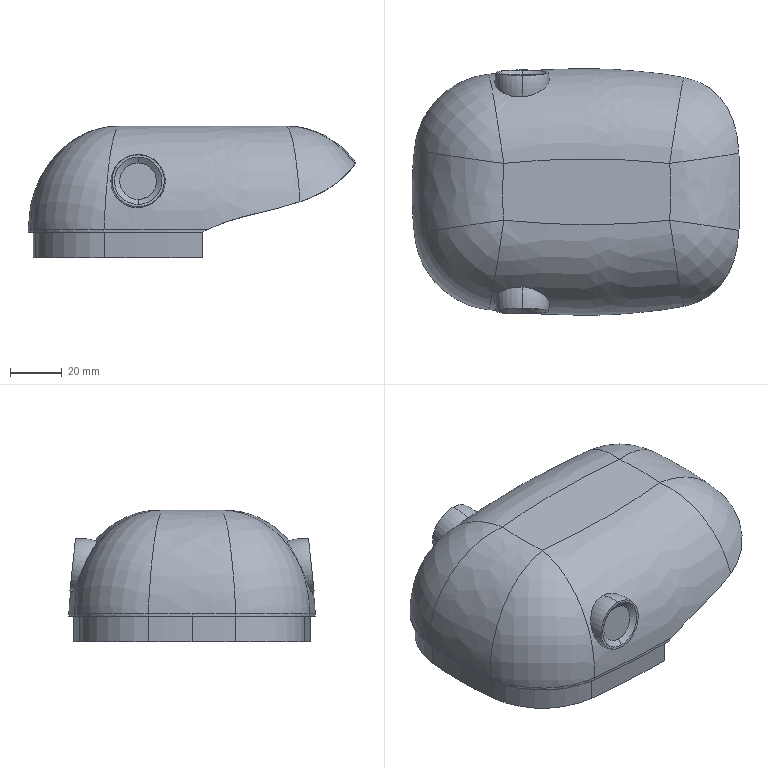Part | SolidWorks | features DelFace 2, Cut 1, Extrusion 1, Fillet 1, ICE 1, MirrorPattern 1, Revolution 1, Shell 1 | 2 solids | 64 faces | box 126.879 x 95.425 x 51 mm | volume 71038 mm3 | cylinder 24 | spline 19 | plane 13 | cone 4 | torus 4 | commonest cylinder face diameters 56.507 x2 56.592 x2 60.592 x2 64.592 x2 303.676 x2 303.761 x2